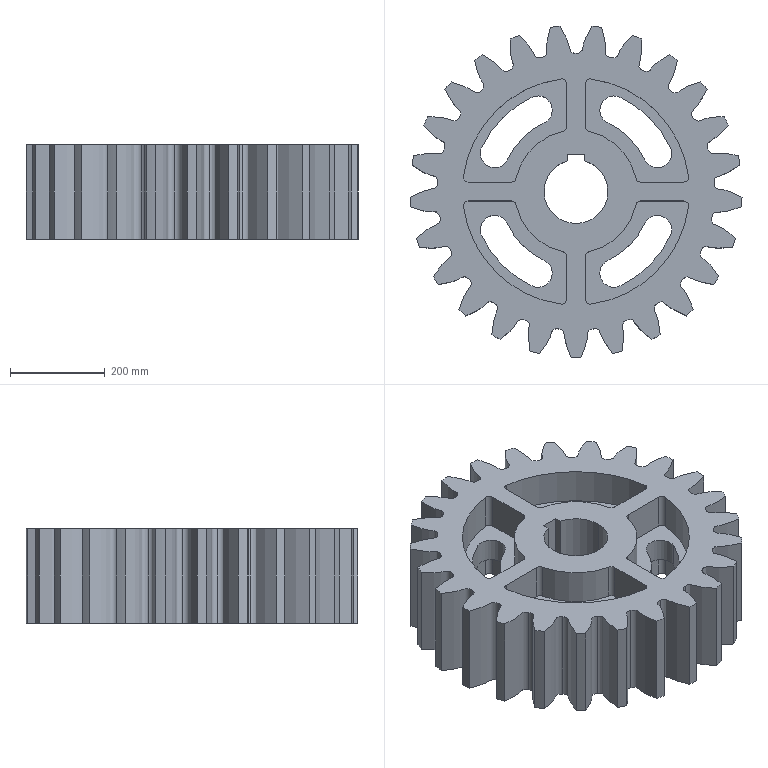Part | NX | features BREP 1 | 1 solid | 179 faces | box 701.605 x 700.371 x 200 mm | volume 42253808 mm3 | cylinder 100 | spline 50 | plane 29 | commonest cylinder face diameters 20 x36 702 x25 60 x12 260 x8 480 x8 320 x4